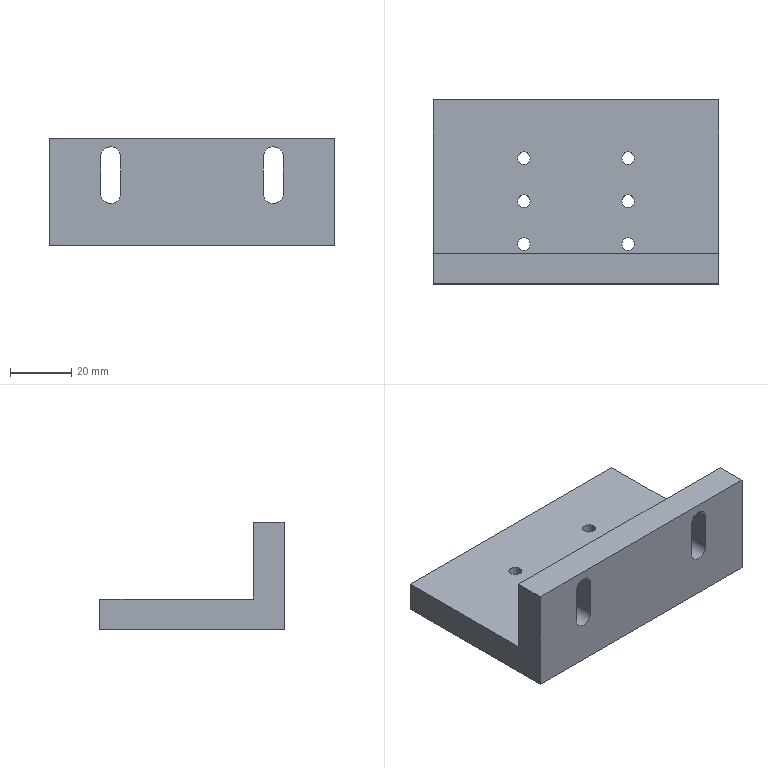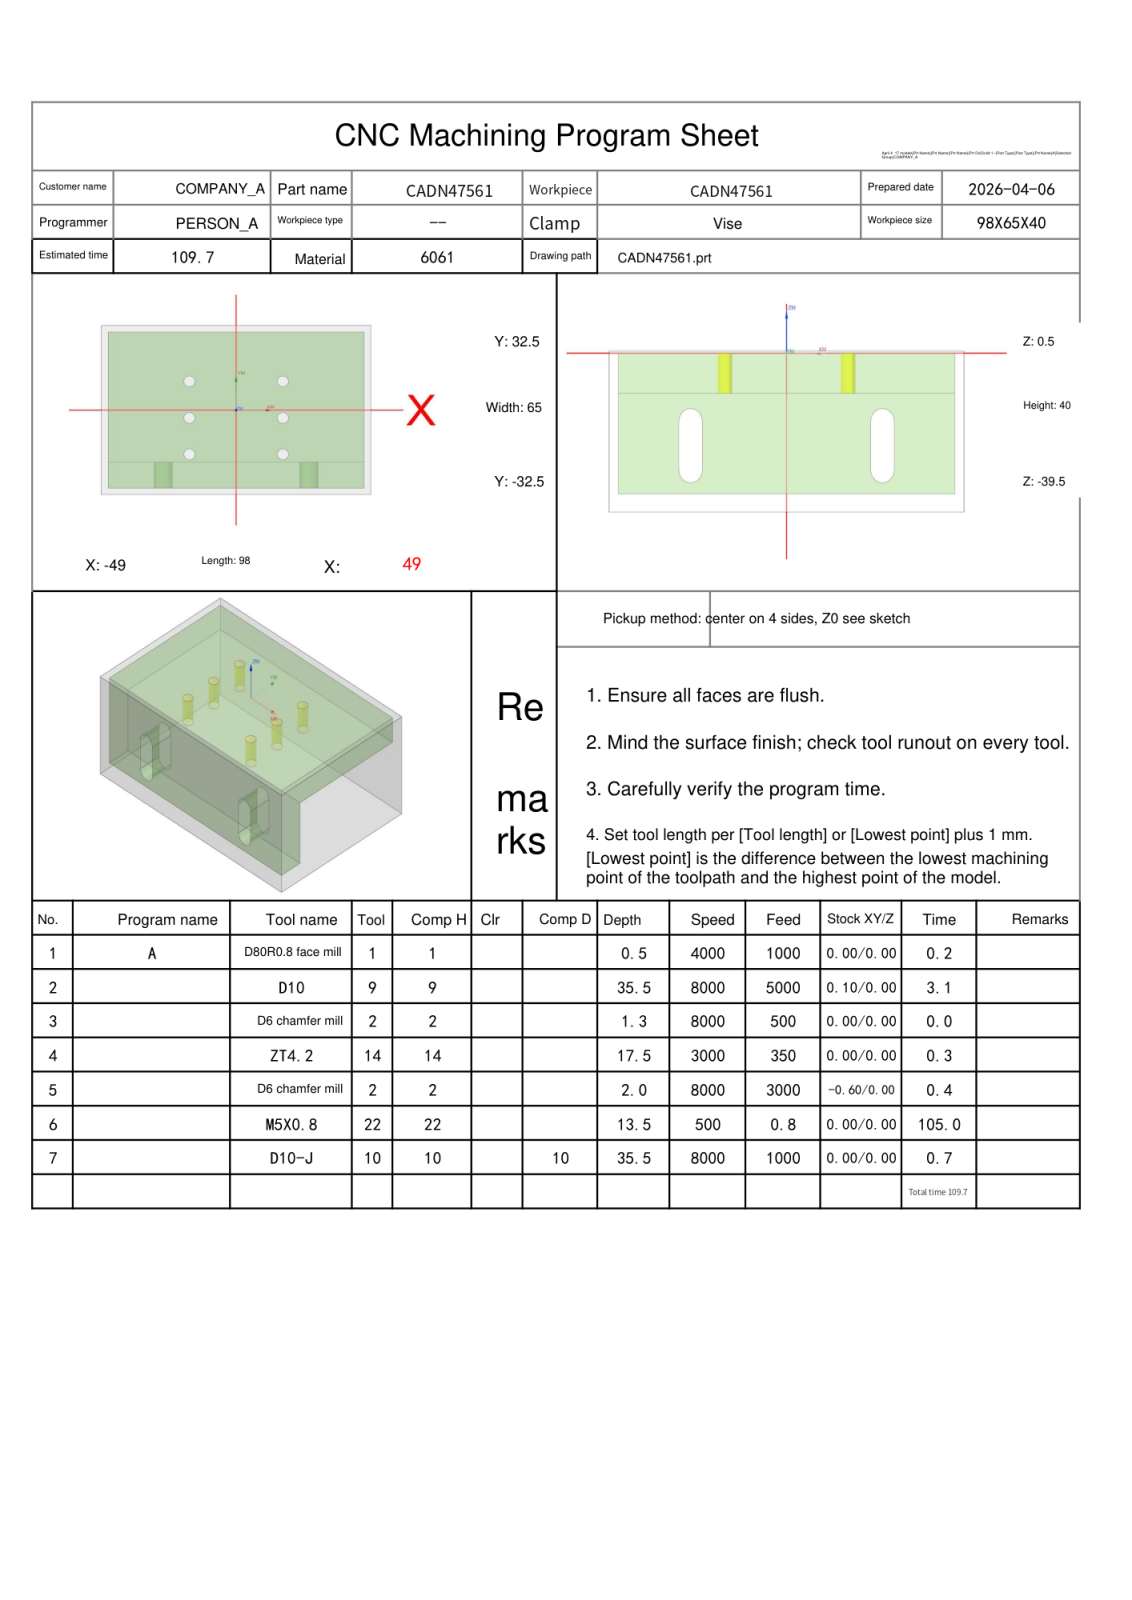NC program | NX | posted by the shop | part box 93 x 60 x 35 mm
Whole program:
%
O0001
(Machine time: 208.64 MIN)
(===Total Tool:6===)
(T1=D80R0.8 face mill D=80.  R=0.8  D-  H01 Z=0.    )
(T9=D10     D=10.  R=0.   D-  H09 Z=-35.  )
(T2=D6 chamfer mill   D=6.   R=0.   D-  H02 Z=-1.5  )
(T14=ZT4.2  D=4.2  DR_a=118 D-  H14 Z=-17.  )
(T22=M5X0.8 D=4.2  DR_a=180 D-  H22 Z=-13.  )
(T10=D10-J  D=10.  R=0.   D10 H10 Z=-35.  )
G80 G90 G17 G49 G40
G91 G28 Z0
M01
N1 T01 M06
(D80R0.8 face mill  D=80. R=0.8 H=01 ce=0.00 di=0.00)
G00 G90 G54 X-91.5 Y0.0 M03 S4000
G43 H01 Z20.
M08
Z2.
G01 Z0.0 F1000.
X-86.5
X86.5
X91.5
Z2.
G00 Z20.
G91 G28 Z0.0
M05
M09
G91 G28 Z0.0
M01
N2 T09 M06
(D10  D=10. R=0. H=09 ce=0.10 di=0.00)
G00 G90 G54 X0.0 Y35.1 M03 S8000
G43 H09 Z20.
M08
Z.5
G01 X46.5 Z.391 F5000.
G02 X51.6 Y30. Z.373 I0.0 J-5.1
G01 Y-30. Z.233
G02 X46.5 Y-35.1 Z.214 I-5.1 J0.0
G01 X-46.5 Z-.003
G02 X-51.6 Y-30. Z-.022 I0.0 J5.1
G01 Y30. Z-.162
G02 X-46.5 Y35.1 Z-.18 I5.1 J0.0
G01 X46.5 Z-.397
G02 X51.6 Y30. Z-.416 I0.0 J-5.1
G01 Y-30. Z-.556
G02 X46.5 Y-35.1 Z-.575 I-5.1 J0.0
G01 X-46.5 Z-.792
G02 X-51.6 Y-30. Z-.811 I0.0 J5.1
G01 Y30. Z-.951
G02 X-46.5 Y35.1 Z-.969 I5.1 J0.0
G01 X46.5 Z-1.186
G02 X51.6 Y30. Z-1.205 I0.0 J-5.1
G01 Y-30. Z-1.345
G02 X46.5 Y-35.1 Z-1.364 I-5.1 J0.0
G01 X-46.5 Z-1.581
G02 X-51.6 Y-30. Z-1.599 I0.0 J5.1
G01 Y30. Z-1.739
G02 X-46.5 Y35.1 Z-1.758 I5.1 J0.0
G01 X46.5 Z-1.975
G02 X51.6 Y30. Z-1.994 I0.0 J-5.1
G01 Y-30. Z-2.134
G02 X46.5 Y-35.1 Z-2.153 I-5.1 J0.0
G01 X-46.5 Z-2.37
G02 X-51.6 Y-30. Z-2.388 I0.0 J5.1
G01 Y30. Z-2.528
G02 X-46.5 Y35.1 Z-2.547 I5.1 J0.0
G01 X46.5 Z-2.764
G02 X51.6 Y30. Z-2.783 I0.0 J-5.1
G01 Y-30. Z-2.923
G02 X46.5 Y-35.1 Z-2.941 I-5.1 J0.0
G01 X-46.5 Z-3.159
G02 X-51.6 Y-30. Z-3.177 I0.0 J5.1
G01 Y30. Z-3.317
G02 X-46.5 Y35.1 Z-3.336 I5.1 J0.0
G01 X46.5 Z-3.553
G02 X51.6 Y30. Z-3.572 I0.0 J-5.1
G01 Y-30. Z-3.712
G02 X46.5 Y-35.1 Z-3.73 I-5.1 J0.0
G01 X-46.5 Z-3.947
G02 X-51.6 Y-30. Z-3.966 I0.0 J5.1
G01 Y30. Z-4.106
G02 X-46.5 Y35.1 Z-4.125 I5.1 J0.0
G01 X46.5 Z-4.342
G02 X51.6 Y30. Z-4.361 I0.0 J-5.1
G01 Y-30. Z-4.501
G02 X46.5 Y-35.1 Z-4.519 I-5.1 J0.0
G01 X-46.5 Z-4.736
G02 X-51.6 Y-30. Z-4.755 I0.0 J5.1
G01 Y30. Z-4.895
G02 X-46.5 Y35.1 Z-4.914 I5.1 J0.0
G01 X46.5 Z-5.131
G02 X51.6 Y30. Z-5.149 I0.0 J-5.1
G01 Y-30. Z-5.289
G02 X46.5 Y-35.1 Z-5.308 I-5.1 J0.0
G01 X-46.5 Z-5.525
G02 X-51.6 Y-30. Z-5.544 I0.0 J5.1
G01 Y30. Z-5.684
G02 X-46.5 Y35.1 Z-5.703 I5.1 J0.0
G01 X46.5 Z-5.92
G02 X51.6 Y30. Z-5.938 I0.0 J-5.1
G01 Y-30. Z-6.078
G02 X46.5 Y-35.1 Z-6.097 I-5.1 J0.0
G01 X-46.5 Z-6.314
G02 X-51.6 Y-30. Z-6.333 I0.0 J5.1
G01 Y30. Z-6.473
G02 X-46.5 Y35.1 Z-6.491 I5.1 J0.0
G01 X46.5 Z-6.709
G02 X51.6 Y30. Z-6.727 I0.0 J-5.1
G01 Y-30. Z-6.867
G02 X46.5 Y-35.1 Z-6.886 I-5.1 J0.0
G01 X-46.5 Z-7.103
G02 X-51.6 Y-30. Z-7.122 I0.0 J5.1
G01 Y30. Z-7.262
G02 X-46.5 Y35.1 Z-7.28 I5.1 J0.0
G01 X46.5 Z-7.497
G02 X51.6 Y30. Z-7.516 I0.0 J-5.1
G01 Y-30. Z-7.656
G02 X46.5 Y-35.1 Z-7.675 I-5.1 J0.0
G01 X-46.5 Z-7.892
G02 X-51.6 Y-30. Z-7.911 I0.0 J5.1
G01 Y30. Z-8.051
G02 X-46.5 Y35.1 Z-8.069 I5.1 J0.0
G01 X46.5 Z-8.286
G02 X51.6 Y30. Z-8.305 I0.0 J-5.1
G01 Y-30. Z-8.445
G02 X46.5 Y-35.1 Z-8.464 I-5.1 J0.0
G01 X-46.5 Z-8.681
G02 X-51.6 Y-30. Z-8.699 I0.0 J5.1
G01 Y30. Z-8.839
G02 X-46.5 Y35.1 Z-8.858 I5.1 J0.0
G01 X46.5 Z-9.075
G02 X51.6 Y30. Z-9.094 I0.0 J-5.1
G01 Y-30. Z-9.234
G02 X46.5 Y-35.1 Z-9.253 I-5.1 J0.0
G01 X-46.5 Z-9.47
G02 X-51.6 Y-30. Z-9.488 I0.0 J5.1
G01 Y30. Z-9.628
G02 X-46.5 Y35.1 Z-9.647 I5.1 J0.0
G01 X46.5 Z-9.864
G02 X51.6 Y30. Z-9.883 I0.0 J-5.1
G01 Y-30. Z-10.023
G02 X46.5 Y-35.1 Z-10.041 I-5.1 J0.0
G01 X-46.5 Z-10.259
G02 X-51.6 Y-30. Z-10.277 I0.0 J5.1
G01 Y30. Z-10.417
G02 X-46.5 Y35.1 Z-10.436 I5.1 J0.0
G01 X46.5 Z-10.653
G02 X51.6 Y30. Z-10.672 I0.0 J-5.1
G01 Y-30. Z-10.812
G02 X46.5 Y-35.1 Z-10.83 I-5.1 J0.0
G01 X-46.5 Z-11.047
G02 X-51.6 Y-30. Z-11.066 I0.0 J5.1
G01 Y30. Z-11.206
G02 X-46.5 Y35.1 Z-11.225 I5.1 J0.0
G01 X46.5 Z-11.442
G02 X51.6 Y30. Z-11.461 I0.0 J-5.1
G01 Y-30. Z-11.601
G02 X46.5 Y-35.1 Z-11.619 I-5.1 J0.0
G01 X-46.5 Z-11.836
G02 X-51.6 Y-30. Z-11.855 I0.0 J5.1
G01 Y30. Z-11.995
G02 X-46.5 Y35.1 Z-12.014 I5.1 J0.0
G01 X46.5 Z-12.231
G02 X51.6 Y30. Z-12.249 I0.0 J-5.1
G01 Y-30. Z-12.389
G02 X46.5 Y-35.1 Z-12.408 I-5.1 J0.0
G01 X-46.5 Z-12.625
G02 X-51.6 Y-30. Z-12.644 I0.0 J5.1
G01 Y30. Z-12.784
G02 X-46.5 Y35.1 Z-12.803 I5.1 J0.0
G01 X46.5 Z-13.02
G02 X51.6 Y30. Z-13.038 I0.0 J-5.1
G01 Y-30. Z-13.178
G02 X46.5 Y-35.1 Z-13.197 I-5.1 J0.0
G01 X-46.5 Z-13.414
G02 X-51.6 Y-30. Z-13.433 I0.0 J5.1
G01 Y30. Z-13.573
G02 X-46.5 Y35.1 Z-13.591 I5.1 J0.0
G01 X46.5 Z-13.809
G02 X51.6 Y30. Z-13.827 I0.0 J-5.1
G01 Y-30. Z-13.967
G02 X46.5 Y-35.1 Z-13.986 I-5.1 J0.0
G01 X-46.5 Z-14.203
G02 X-51.6 Y-30. Z-14.222 I0.0 J5.1
G01 Y30. Z-14.362
G02 X-46.5 Y35.1 Z-14.38 I5.1 J0.0
G01 X46.5 Z-14.597
G02 X51.6 Y30. Z-14.616 I0.0 J-5.1
G01 Y-30. Z-14.756
G02 X46.5 Y-35.1 Z-14.775 I-5.1 J0.0
G01 X-46.5 Z-14.992
G02 X-51.6 Y-30. Z-15.011 I0.0 J5.1
G01 Y30. Z-15.151
G02 X-46.5 Y35.1 Z-15.169 I5.1 J0.0
G01 X46.5 Z-15.386
G02 X51.6 Y30. Z-15.405 I0.0 J-5.1
G01 Y-30. Z-15.545
G02 X46.5 Y-35.1 Z-15.564 I-5.1 J0.0
G01 X-46.5 Z-15.781
G02 X-51.6 Y-30. Z-15.799 I0.0 J5.1
G01 Y30. Z-15.939
G02 X-46.5 Y35.1 Z-15.958 I5.1 J0.0
G01 X46.5 Z-16.175
G02 X51.6 Y30. Z-16.194 I0.0 J-5.1
G01 Y-30. Z-16.334
G02 X46.5 Y-35.1 Z-16.353 I-5.1 J0.0
G01 X-46.5 Z-16.57
G02 X-51.6 Y-30. Z-16.588 I0.0 J5.1
G01 Y30. Z-16.728
G02 X-46.5 Y35.1 Z-16.747 I5.1 J0.0
G01 X46.5 Z-16.964
G02 X51.6 Y30. Z-16.983 I0.0 J-5.1
G01 Y-30. Z-17.123
G02 X46.5 Y-35.1 Z-17.141 I-5.1 J0.0
G01 X-46.5 Z-17.359
G02 X-51.6 Y-30. Z-17.377 I0.0 J5.1
G01 Y30. Z-17.517
G02 X-46.5 Y35.1 Z-17.536 I5.1 J0.0
G01 X46.5 Z-17.753
G02 X51.6 Y30. Z-17.772 I0.0 J-5.1
G01 Y-30. Z-17.912
G02 X46.5 Y-35.1 Z-17.93 I-5.1 J0.0
G01 X-46.5 Z-18.147
G02 X-51.6 Y-30. Z-18.166 I0.0 J5.1
G01 Y30. Z-18.306
G02 X-46.5 Y35.1 Z-18.325 I5.1 J0.0
G01 X46.5 Z-18.542
G02 X51.6 Y30. Z-18.561 I0.0 J-5.1
G01 Y-30. Z-18.701
G02 X46.5 Y-35.1 Z-18.719 I-5.1 J0.0
G01 X-46.5 Z-18.936
G02 X-51.6 Y-30. Z-18.955 I0.0 J5.1
G01 Y30. Z-19.095
G02 X-46.5 Y35.1 Z-19.114 I5.1 J0.0
G01 X46.5 Z-19.331
G02 X51.6 Y30. Z-19.349 I0.0 J-5.1
G01 Y-30. Z-19.489
G02 X46.5 Y-35.1 Z-19.508 I-5.1 J0.0
G01 X-46.5 Z-19.725
G02 X-51.6 Y-30. Z-19.744 I0.0 J5.1
G01 Y30. Z-19.884
G02 X-46.5 Y35.1 Z-19.903 I5.1 J0.0
G01 X46.5 Z-20.12
G02 X51.6 Y30. Z-20.138 I0.0 J-5.1
G01 Y-30. Z-20.278
G02 X46.5 Y-35.1 Z-20.297 I-5.1 J0.0
G01 X-46.5 Z-20.514
G02 X-51.6 Y-30. Z-20.533 I0.0 J5.1
G01 Y30. Z-20.673
G02 X-46.5 Y35.1 Z-20.691 I5.1 J0.0
G01 X46.5 Z-20.909
G02 X51.6 Y30. Z-20.927 I0.0 J-5.1
G01 Y-30. Z-21.067
G02 X46.5 Y-35.1 Z-21.086 I-5.1 J0.0
G01 X-46.5 Z-21.303
G02 X-51.6 Y-30. Z-21.322 I0.0 J5.1
G01 Y30. Z-21.462
G02 X-46.5 Y35.1 Z-21.48 I5.1 J0.0
G01 X46.5 Z-21.697
G02 X51.6 Y30. Z-21.716 I0.0 J-5.1
G01 Y-30. Z-21.856
G02 X46.5 Y-35.1 Z-21.875 I-5.1 J0.0
G01 X-46.5 Z-22.092
G02 X-51.6 Y-30. Z-22.111 I0.0 J5.1
G01 Y30. Z-22.251
G02 X-46.5 Y35.1 Z-22.269 I5.1 J0.0
G01 X46.5 Z-22.486
G02 X51.6 Y30. Z-22.505 I0.0 J-5.1
G01 Y-30. Z-22.645
G02 X46.5 Y-35.1 Z-22.664 I-5.1 J0.0
G01 X-46.5 Z-22.881
G02 X-51.6 Y-30. Z-22.899 I0.0 J5.1
G01 Y30. Z-23.039
G02 X-46.5 Y35.1 Z-23.058 I5.1 J0.0
G01 X46.5 Z-23.275
G02 X51.6 Y30. Z-23.294 I0.0 J-5.1
G01 Y-30. Z-23.434
G02 X46.5 Y-35.1 Z-23.453 I-5.1 J0.0
G01 X-46.5 Z-23.67
G02 X-51.6 Y-30. Z-23.688 I0.0 J5.1
G01 Y30. Z-23.828
G02 X-46.5 Y35.1 Z-23.847 I5.1 J0.0
G01 X46.5 Z-24.064
G02 X51.6 Y30. Z-24.083 I0.0 J-5.1
G01 Y-30. Z-24.223
G02 X46.5 Y-35.1 Z-24.241 I-5.1 J0.0
G01 X-46.5 Z-24.459
G02 X-51.6 Y-30. Z-24.477 I0.0 J5.1
G01 Y30. Z-24.617
G02 X-46.5 Y35.1 Z-24.636 I5.1 J0.0
G01 X46.5 Z-24.853
G02 X51.6 Y30. Z-24.872 I0.0 J-5.1
G01 Y-30. Z-25.012
G02 X46.5 Y-35.1 Z-25.03 I-5.1 J0.0
G01 X-46.5 Z-25.247
G02 X-51.6 Y-30. Z-25.266 I0.0 J5.1
G01 Y30. Z-25.406
G02 X-46.5 Y35.1 Z-25.425 I5.1 J0.0
G01 X46.5 Z-25.642
G02 X51.6 Y30. Z-25.661 I0.0 J-5.1
G01 Y-30. Z-25.801
G02 X46.5 Y-35.1 Z-25.819 I-5.1 J0.0
G01 X-46.5 Z-26.036
G02 X-51.6 Y-30. Z-26.055 I0.0 J5.1
G01 Y30. Z-26.195
G02 X-46.5 Y35.1 Z-26.214 I5.1 J0.0
G01 X46.5 Z-26.431
G02 X51.6 Y30. Z-26.449 I0.0 J-5.1
G01 Y-30. Z-26.589
G02 X46.5 Y-35.1 Z-26.608 I-5.1 J0.0
G01 X-46.5 Z-26.825
G02 X-51.6 Y-30. Z-26.844 I0.0 J5.1
G01 Y30. Z-26.984
G02 X-46.5 Y35.1 Z-27.003 I5.1 J0.0
G01 X46.5 Z-27.22
G02 X51.6 Y30. Z-27.238 I0.0 J-5.1
G01 Y-30. Z-27.378
G02 X46.5 Y-35.1 Z-27.397 I-5.1 J0.0
G01 X-46.5 Z-27.614
G02 X-51.6 Y-30. Z-27.633 I0.0 J5.1
G01 Y30. Z-27.773
G02 X-46.5 Y35.1 Z-27.791 I5.1 J0.0
G01 X46.5 Z-28.009
G02 X51.6 Y30. Z-28.027 I0.0 J-5.1
G01 Y-30. Z-28.167
G02 X46.5 Y-35.1 Z-28.186 I-5.1 J0.0
G01 X-46.5 Z-28.403
G02 X-51.6 Y-30. Z-28.422 I0.0 J5.1
G01 Y30. Z-28.562
G02 X-46.5 Y35.1 Z-28.58 I5.1 J0.0
G01 X46.5 Z-28.797
G02 X51.6 Y30. Z-28.816 I0.0 J-5.1
G01 Y-30. Z-28.956
G02 X46.5 Y-35.1 Z-28.975 I-5.1 J0.0
G01 X-46.5 Z-29.192
G02 X-51.6 Y-30. Z-29.211 I0.0 J5.1
G01 Y30. Z-29.351
G02 X-46.5 Y35.1 Z-29.369 I5.1 J0.0
G01 X46.5 Z-29.586
G02 X51.6 Y30. Z-29.605 I0.0 J-5.1
G01 Y-30. Z-29.745
G02 X46.5 Y-35.1 Z-29.764 I-5.1 J0.0
G01 X-46.5 Z-29.981
G02 X-51.6 Y-30. Z-29.999 I0.0 J5.1
G01 Y30. Z-30.139
G02 X-46.5 Y35.1 Z-30.158 I5.1 J0.0
G01 X46.5 Z-30.375
G02 X51.6 Y30. Z-30.394 I0.0 J-5.1
G01 Y-30. Z-30.534
G02 X46.5 Y-35.1 Z-30.553 I-5.1 J0.0
G01 X-46.5 Z-30.77
G02 X-51.6 Y-30. Z-30.788 I0.0 J5.1
G01 Y30. Z-30.928
G02 X-46.5 Y35.1 Z-30.947 I5.1 J0.0
G01 X46.5 Z-31.164
G02 X51.6 Y30. Z-31.183 I0.0 J-5.1
G01 Y-30. Z-31.323
G02 X46.5 Y-35.1 Z-31.341 I-5.1 J0.0
G01 X-46.5 Z-31.559
G02 X-51.6 Y-30. Z-31.577 I0.0 J5.1
G01 Y30. Z-31.717
G02 X-46.5 Y35.1 Z-31.736 I5.1 J0.0
G01 X46.5 Z-31.953
G02 X51.6 Y30. Z-31.972 I0.0 J-5.1
G01 Y-30. Z-32.112
G02 X46.5 Y-35.1 Z-32.13 I-5.1 J0.0
G01 X-46.5 Z-32.347
G02 X-51.6 Y-30. Z-32.366 I0.0 J5.1
G01 Y30. Z-32.506
G02 X-46.5 Y35.1 Z-32.525 I5.1 J0.0
G01 X46.5 Z-32.742
G02 X51.6 Y30. Z-32.761 I0.0 J-5.1
G01 Y-30. Z-32.901
G02 X46.5 Y-35.1 Z-32.919 I-5.1 J0.0
G01 X-46.5 Z-33.136
G02 X-51.6 Y-30. Z-33.155 I0.0 J5.1
G01 Y30. Z-33.295
G02 X-46.5 Y35.1 Z-33.314 I5.1 J0.0
G01 X46.5 Z-33.531
G02 X51.6 Y30. Z-33.549 I0.0 J-5.1
G01 Y-30. Z-33.689
G02 X46.5 Y-35.1 Z-33.708 I-5.1 J0.0
G01 X-46.5 Z-33.925
G02 X-51.6 Y-30. Z-33.944 I0.0 J5.1
G01 Y30. Z-34.084
G02 X-46.5 Y35.1 Z-34.103 I5.1 J0.0
G01 X46.5 Z-34.32
G02 X51.6 Y30. Z-34.338 I0.0 J-5.1
G01 Y-30. Z-34.478
G02 X46.5 Y-35.1 Z-34.497 I-5.1 J0.0
G01 X-46.5 Z-34.714
G02 X-51.6 Y-30. Z-34.733 I0.0 J5.1
G01 Y30. Z-34.873
G02 X-46.5 Y35.1 Z-34.891 I5.1 J0.0
G01 X0.0 Z-35.
X46.5
G02 X51.6 Y30. I0.0 J-5.1
G01 Y-30.
G02 X46.5 Y-35.1 I-5.1 J0.0
G01 X-46.5
G02 X-51.6 Y-30. I0.0 J5.1
G01 Y30.
G02 X-46.5 Y35.1 I5.1 J0.0
G01 X0.0
X.5
Z-34.
G00 Z20.
G91 G28 Z0.0
M05
M09
G91 G28 Z0.0
M01
N3 T02 M06
(D6 chamfer mill  D=6. R=0. H=02 ce=0.00 di=0.00)
G00 G90 G54 X17. Y-17. M03 S8000
G43 H02 Z20.
M08
G98 G81 X17. Y-17. Z-.8 R1. F500.
Y-3.
Y11.
X-17.
Y-3.
Y-17.
G80
G00 Z20.
G91 G28 Z0.0
M05
M09
G91 G28 Z0.0
M01
N4 T14 M06
(ZT4.2 D=4.2 DR_a=118 H=14)
G00 G90 G54 X17. Y-17. M03 S3000
G43 H14 Z20.
M08
G98 G83 X17. Y-17. Z-17. R1. F350. Q3.
Y-3.
Y11.
X-17.
Y-3.
Y-17.
G80
G00 Z20.
G91 G28 Z0.0
M05
M09
G91 G28 Z0.0
M01
N5 T02 M06
(D6 chamfer mill  D=6. R=0. H=02 ce=0.00 di=0.00)
G00 G90 G54 X.25 Y-32.128 M03 S8000
G43 H02 Z20.
M08
Z2.099
G01 Z-1.5 F3000.
G03 X.33 Y-31.828 I-.52 J.3
X.03 Y-31.308 I-.6 J0.0
G01 X0.0 Y-31.3
X-46.5
G02 X-47.8 Y-30. I0.0 J1.3
G01 Y30.
G02 X-46.5 Y31.3 I1.3 J0.0
G01 X46.5
G02 X47.8 Y30. I0.0 J-1.3
G01 Y-30.
G02 X46.5 Y-31.3 I-1.3 J0.0
G01 X0.0
X-.03 Y-31.308
G03 X-.33 Y-31.828 I.3 J-.52
X-.25 Y-32.128 I.6 J0.0
G01 Z2.099
G00 Z20.
G00 G90 X-16.926 Y10.337 M03 S8000
Z20.
Z-.5
G01 Z-1. F500.
X-16.833 Y9.5
G03 X-15.333 Y11. I0.0 J1.5
X-17. Y12.667 I-1.667 J0.0
X-18.667 Y11. I0.0 J-1.667
X-17. Y9.333 I1.667 J0.0
X-15.333 Y11. I0.0 J1.667
X-16.833 Y12.5 I-1.5 J0.0
G01 X-16.926 Y11.663
Z-.5
G00 Z20.
Y-3.663
Z-.5
G01 Z-1.
X-16.833 Y-4.5
G03 X-15.333 Y-3. I0.0 J1.5
X-17. Y-1.333 I-1.667 J0.0
X-18.667 Y-3. I0.0 J-1.667
X-17. Y-4.667 I1.667 J0.0
X-15.333 Y-3. I0.0 J1.667
X-16.833 Y-1.5 I-1.5 J0.0
G01 X-16.926 Y-2.337
Z-.5
G00 Z20.
Y-17.663
Z-.5
G01 Z-1.
X-16.833 Y-18.5
G03 X-15.333 Y-17. I0.0 J1.5
X-17. Y-15.333 I-1.667 J0.0
X-18.667 Y-17. I0.0 J-1.667
X-17. Y-18.667 I1.667 J0.0
X-15.333 Y-17. I0.0 J1.667
X-16.833 Y-15.5 I-1.5 J0.0
G01 X-16.926 Y-16.337
Z-.5
G00 Z20.
X17.074 Y-17.663
Z-.5
G01 Z-1.
X17.167 Y-18.5
G03 X18.667 Y-17. I0.0 J1.5
X17. Y-15.333 I-1.667 J0.0
X15.333 Y-17. I0.0 J-1.667
X17. Y-18.667 I1.667 J0.0
X18.667 Y-17. I0.0 J1.667
X17.167 Y-15.5 I-1.5 J0.0
G01 X17.074 Y-16.337
Z-.5
G00 Z20.
Y-3.663
Z-.5
G01 Z-1.
X17.167 Y-4.5
G03 X18.667 Y-3. I0.0 J1.5
X17. Y-1.333 I-1.667 J0.0
X15.333 Y-3. I0.0 J-1.667
X17. Y-4.667 I1.667 J0.0
X18.667 Y-3. I0.0 J1.667
X17.167 Y-1.5 I-1.5 J0.0
G01 X17.074 Y-2.337
Z-.5
G00 Z20.
Y10.337
Z-.5
G01 Z-1.
X17.167 Y9.5
G03 X18.667 Y11. I0.0 J1.5
X17. Y12.667 I-1.667 J0.0
X15.333 Y11. I0.0 J-1.667
X17. Y9.333 I1.667 J0.0
X18.667 Y11. I0.0 J1.667
X17.167 Y12.5 I-1.5 J0.0
G01 X17.074 Y11.663
Z-.5
G00 Z20.
G91 G28 Z0.0
M05
M09
G91 G28 Z0.0
M01
N6 T22 M06
(M5X0.8 D=4.2 DR_a=180 H=22)
G00 G90 G54 X17. Y-17. M03 S500
G43 H22 Z20.
M08
G95
G98 G84 X17. Y-17. Z-13. R1. F.8 Q3.
Y-3.
Y11.
X-17.
Y-3.
Y-17.
G80
G94
G00 Z20.
G91 G28 Z0.0
M05
M09
G91 G28 Z0.0
M01
N7 T10 M06
(D10-J  D=10. R=0. H=10 ce=0.00 di=0.00)
G00 G90 G54 X47.513 Y-36.116 M03 S8000
G43 H10 Z20.
M08
Z-17.
G01 Z-17.5 F1000.
G41 D10
X47.497 Y-35.917
G03 X46.5 Y-35. I-.997 J-.083
G01 X-46.5
G02 X-51.5 Y-30. I0.0 J5.
G01 Y30.
G02 X-46.5 Y35. I5. J0.0
G01 X46.5
G02 X51.5 Y30. I0.0 J-5.
G01 Y-30.
G02 X46.5 Y-35. I-5. J0.0
G01 X46.
G03 X45. Y-36. I0.0 J-1.
G01 G40 Y-36.2
Z-17.
G00 Z20.
X47.513 Y-36.116
Z-34.5
G01 Z-35.
G41 D10
X47.497 Y-35.917
G03 X46.5 Y-35. I-.997 J-.083
G01 X-46.5
G02 X-51.5 Y-30. I0.0 J5.
G01 Y30.
G02 X-46.5 Y35. I5. J0.0
G01 X46.5
G02 X51.5 Y30. I0.0 J-5.
G01 Y-30.
G02 X46.5 Y-35. I-5. J0.0
G01 X46.
G03 X45. Y-36. I0.0 J-1.
G01 G40 Y-36.2
Z-34.5
G00 Z20.
M05
M09
G91 G28 Z0.0
G91 G28 Y0.0
M30
%